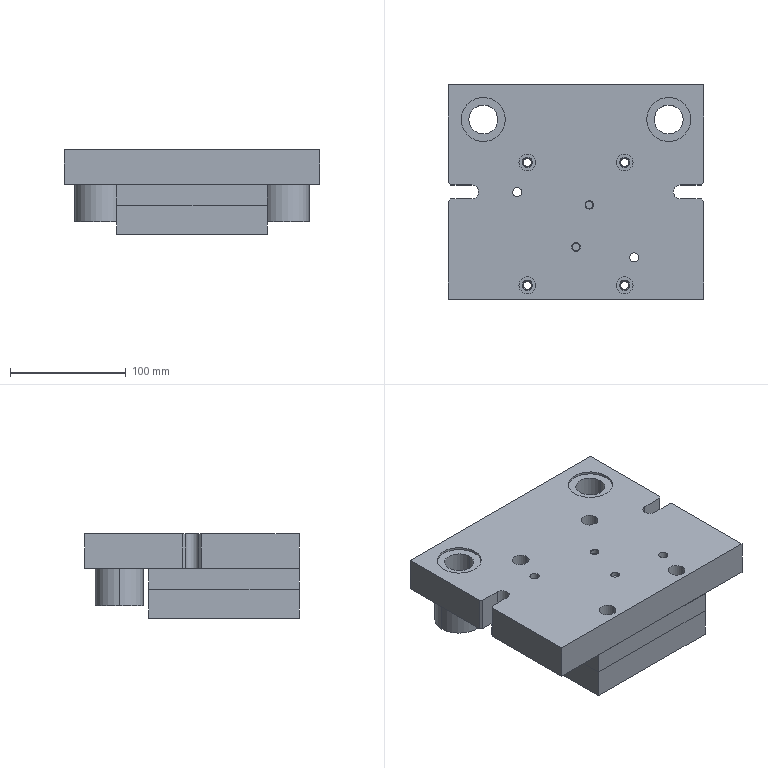Part | SolidWorks | 12 solids | 237 faces | box 220 x 185 x 73 mm | volume 1914811 mm3 | cylinder 109 | plane 82 | cone 22 | spline 20 | torus 4 | commonest cylinder face diameters 9.007 x16 8 x12 6 x8 6.805 x8 6.806 x8 14.5 x8